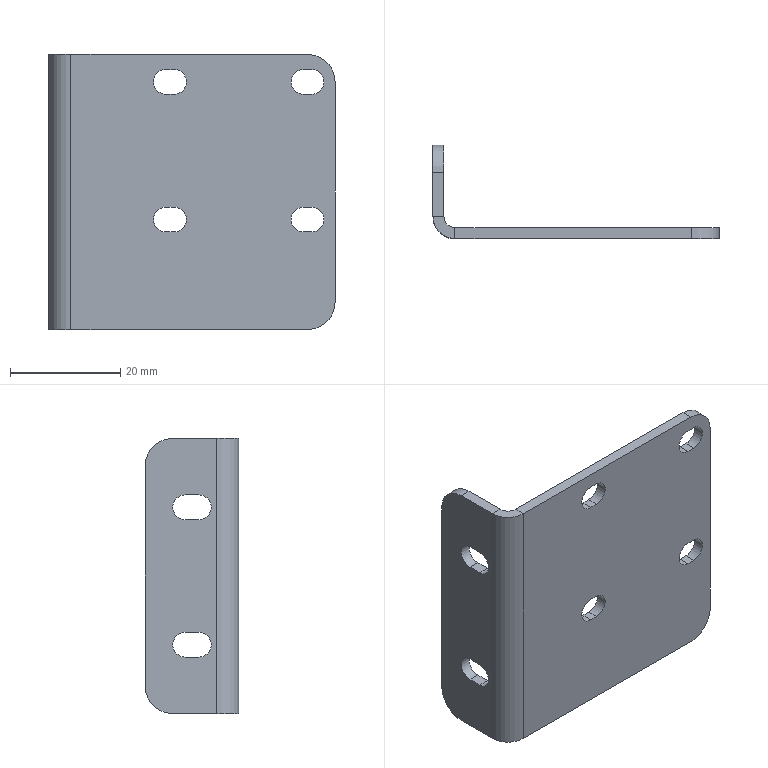Part | SolidWorks | features HoleWzd 2, Fillet 1, FlatPattern 1, SMBaseFlange 1, SheetMetal 1 | 1 solid | 42 faces | box 52 x 17 x 50 mm | volume 6238 mm3 | plane 24 | cylinder 18 | commonest cylinder face diameters 4.5 x12 10 x4 4 x1 8 x1
STEP:
#1=CARTESIAN_POINT('',(0.,-13.,50.));
#2=VERTEX_POINT('',#1);
#3=CARTESIAN_POINT('',(2.,-13.,50.));
#4=VERTEX_POINT('',#3);
#5=CARTESIAN_POINT('',(0.,-13.,50.));
#6=DIRECTION('',(1.,0.,0.));
#7=VECTOR('',#6,1000.);
#8=LINE('',#5,#7);
#9=EDGE_CURVE('',#2,#4,#8,.T.);
#10=ORIENTED_EDGE('',*,*,#9,.F.);
#11=CARTESIAN_POINT('',(4.,-17.,50.));
#12=VERTEX_POINT('',#11);
#13=CARTESIAN_POINT('',(4.,-13.,50.));
#14=DIRECTION('',(0.,0.,1.));
#15=DIRECTION('',(-1.,0.,0.));
#16=AXIS2_PLACEMENT_3D('',#13,#14,#15);
#17=CIRCLE('',#16,4.);
#18=EDGE_CURVE('',#2,#12,#17,.T.);
#19=ORIENTED_EDGE('',*,*,#18,.T.);
#20=CARTESIAN_POINT('',(4.,-15.,50.));
#21=VERTEX_POINT('',#20);
#22=CARTESIAN_POINT('',(4.,-15.,50.));
#23=DIRECTION('',(0.,-1.,0.));
#24=VECTOR('',#23,1000.);
#25=LINE('',#22,#24);
#26=EDGE_CURVE('',#21,#12,#25,.T.);
#27=ORIENTED_EDGE('',*,*,#26,.F.);
#28=CARTESIAN_POINT('',(4.,-13.,50.));
#29=DIRECTION('',(0.,0.,1.));
#30=DIRECTION('',(1.,0.,0.));
#31=AXIS2_PLACEMENT_3D('',#28,#29,#30);
#32=CIRCLE('',#31,2.);
#33=EDGE_CURVE('',#4,#21,#32,.T.);
#34=ORIENTED_EDGE('',*,*,#33,.F.);
#35=EDGE_LOOP('',(#10,#19,#27,#34));
#36=FACE_OUTER_BOUND('',#35,.T.);
#37=CARTESIAN_POINT('',(0.,-13.,50.));
#38=DIRECTION('',(0.,0.,1.));
#39=DIRECTION('',(1.,0.,0.));
#40=AXIS2_PLACEMENT_3D('',#37,#38,#39);
#41=PLANE('',#40);
#42=ADVANCED_FACE('',(#36),#41,.T.);
#43=CARTESIAN_POINT('',(2.,-5.,50.));
#44=VERTEX_POINT('',#43);
#45=CARTESIAN_POINT('',(2.,0.,50.));
#46=DIRECTION('',(0.,-1.,0.));
#47=VECTOR('',#46,1000.);
#48=LINE('',#45,#47);
#49=EDGE_CURVE('',#44,#4,#48,.T.);
#50=ORIENTED_EDGE('',*,*,#49,.F.);
#51=CARTESIAN_POINT('',(0.,-5.,50.));
#52=VERTEX_POINT('',#51);
#53=CARTESIAN_POINT('',(4.,-5.,50.));
#54=DIRECTION('',(-1.,0.,0.));
#55=VECTOR('',#54,1000.);
#56=LINE('',#53,#55);
#57=EDGE_CURVE('',#44,#52,#56,.T.);
#58=ORIENTED_EDGE('',*,*,#57,.T.);
#59=CARTESIAN_POINT('',(0.,0.,50.));
#60=DIRECTION('',(0.,-1.,0.));
#61=VECTOR('',#60,1000.);
#62=LINE('',#59,#61);
#63=EDGE_CURVE('',#52,#2,#62,.T.);
#64=ORIENTED_EDGE('',*,*,#63,.T.);
#65=ORIENTED_EDGE('',*,*,#9,.T.);
#66=EDGE_LOOP('',(#50,#58,#64,#65));
#67=FACE_OUTER_BOUND('',#66,.T.);
#68=CARTESIAN_POINT('',(4.,-15.,50.));
#69=DIRECTION('',(0.,0.,1.));
#70=DIRECTION('',(1.,0.,0.));
#71=AXIS2_PLACEMENT_3D('',#68,#69,#70);
#72=PLANE('',#71);
#73=ADVANCED_FACE('',(#67),#72,.T.);
#74=CARTESIAN_POINT('',(4.,-17.,0.));
#75=VERTEX_POINT('',#74);
#76=CARTESIAN_POINT('',(4.,-15.,0.));
#77=VERTEX_POINT('',#76);
#78=CARTESIAN_POINT('',(4.,-17.,0.));
#79=DIRECTION('',(0.,1.,0.));
#80=VECTOR('',#79,1000.);
#81=LINE('',#78,#80);
#82=EDGE_CURVE('',#75,#77,#81,.T.);
#83=ORIENTED_EDGE('',*,*,#82,.F.);
#84=CARTESIAN_POINT('',(0.,-13.,0.));
#85=VERTEX_POINT('',#84);
#86=CARTESIAN_POINT('',(4.,-13.,0.));
#87=DIRECTION('',(0.,0.,1.));
#88=DIRECTION('',(-1.,0.,0.));
#89=AXIS2_PLACEMENT_3D('',#86,#87,#88);
#90=CIRCLE('',#89,4.);
#91=EDGE_CURVE('',#85,#75,#90,.T.);
#92=ORIENTED_EDGE('',*,*,#91,.F.);
#93=CARTESIAN_POINT('',(2.,-13.,0.));
#94=VERTEX_POINT('',#93);
#95=CARTESIAN_POINT('',(2.,-13.,0.));
#96=DIRECTION('',(-1.,0.,0.));
#97=VECTOR('',#96,1000.);
#98=LINE('',#95,#97);
#99=EDGE_CURVE('',#94,#85,#98,.T.);
#100=ORIENTED_EDGE('',*,*,#99,.F.);
#101=CARTESIAN_POINT('',(4.,-13.,0.));
#102=DIRECTION('',(0.,0.,1.));
#103=DIRECTION('',(1.,0.,0.));
#104=AXIS2_PLACEMENT_3D('',#101,#102,#103);
#105=CIRCLE('',#104,2.);
#106=EDGE_CURVE('',#94,#77,#105,.T.);
#107=ORIENTED_EDGE('',*,*,#106,.T.);
#108=EDGE_LOOP('',(#83,#92,#100,#107));
#109=FACE_OUTER_BOUND('',#108,.T.);
#110=CARTESIAN_POINT('',(4.,-17.,0.));
#111=DIRECTION('',(0.,0.,-1.));
#112=DIRECTION('',(-1.,0.,0.));
#113=AXIS2_PLACEMENT_3D('',#110,#111,#112);
#114=PLANE('',#113);
#115=ADVANCED_FACE('',(#109),#114,.T.);
#116=CARTESIAN_POINT('',(47.,-15.,0.));
#117=VERTEX_POINT('',#116);
#118=CARTESIAN_POINT('',(0.,-15.,0.));
#119=DIRECTION('',(1.,0.,0.));
#120=VECTOR('',#119,1000.);
#121=LINE('',#118,#120);
#122=EDGE_CURVE('',#77,#117,#121,.T.);
#123=ORIENTED_EDGE('',*,*,#122,.T.);
#124=CARTESIAN_POINT('',(47.,-17.,0.));
#125=VERTEX_POINT('',#124);
#126=CARTESIAN_POINT('',(47.,-13.,0.));
#127=DIRECTION('',(0.,-1.,0.));
#128=VECTOR('',#127,1000.);
#129=LINE('',#126,#128);
#130=EDGE_CURVE('',#117,#125,#129,.T.);
#131=ORIENTED_EDGE('',*,*,#130,.T.);
#132=CARTESIAN_POINT('',(0.,-17.,0.));
#133=DIRECTION('',(1.,0.,0.));
#134=VECTOR('',#133,1000.);
#135=LINE('',#132,#134);
#136=EDGE_CURVE('',#75,#125,#135,.T.);
#137=ORIENTED_EDGE('',*,*,#136,.F.);
#138=ORIENTED_EDGE('',*,*,#82,.T.);
#139=EDGE_LOOP('',(#123,#131,#137,#138));
#140=FACE_OUTER_BOUND('',#139,.T.);
#141=CARTESIAN_POINT('',(2.,-13.,0.));
#142=DIRECTION('',(0.,0.,-1.));
#143=DIRECTION('',(-1.,0.,0.));
#144=AXIS2_PLACEMENT_3D('',#141,#142,#143);
#145=PLANE('',#144);
#146=ADVANCED_FACE('',(#140),#145,.T.);
#147=CARTESIAN_POINT('',(46.25,-17.,47.25));
#148=VERTEX_POINT('',#147);
#149=CARTESIAN_POINT('',(47.75,-17.,47.25));
#150=VERTEX_POINT('',#149);
#151=CARTESIAN_POINT('',(46.25,-17.,47.25));
#152=DIRECTION('',(1.,0.,0.));
#153=VECTOR('',#152,1000.);
#154=LINE('',#151,#153);
#155=EDGE_CURVE('',#148,#150,#154,.T.);
#156=ORIENTED_EDGE('',*,*,#155,.T.);
#157=CARTESIAN_POINT('',(47.75,-17.,42.75));
#158=VERTEX_POINT('',#157);
#159=CARTESIAN_POINT('',(47.75,-17.,45.));
#160=DIRECTION('',(0.,1.,0.));
#161=DIRECTION('',(0.,0.,1.));
#162=AXIS2_PLACEMENT_3D('',#159,#160,#161);
#163=CIRCLE('',#162,2.25);
#164=EDGE_CURVE('',#150,#158,#163,.T.);
#165=ORIENTED_EDGE('',*,*,#164,.T.);
#166=CARTESIAN_POINT('',(46.25,-17.,42.75));
#167=VERTEX_POINT('',#166);
#168=CARTESIAN_POINT('',(46.25,-17.,42.75));
#169=DIRECTION('',(1.,0.,0.));
#170=VECTOR('',#169,1000.);
#171=LINE('',#168,#170);
#172=EDGE_CURVE('',#167,#158,#171,.T.);
#173=ORIENTED_EDGE('',*,*,#172,.F.);
#174=CARTESIAN_POINT('',(46.25,-17.,45.));
#175=DIRECTION('',(0.,1.,0.));
#176=DIRECTION('',(0.,0.,1.));
#177=AXIS2_PLACEMENT_3D('',#174,#175,#176);
#178=CIRCLE('',#177,2.25);
#179=EDGE_CURVE('',#167,#148,#178,.T.);
#180=ORIENTED_EDGE('',*,*,#179,.T.);
#181=EDGE_LOOP('',(#156,#165,#173,#180));
#182=FACE_BOUND('',#181,.T.);
#183=CARTESIAN_POINT('',(21.25,-17.,47.25));
#184=VERTEX_POINT('',#183);
#185=CARTESIAN_POINT('',(22.75,-17.,47.25));
#186=VERTEX_POINT('',#185);
#187=CARTESIAN_POINT('',(21.25,-17.,47.25));
#188=DIRECTION('',(1.,0.,0.));
#189=VECTOR('',#188,1000.);
#190=LINE('',#187,#189);
#191=EDGE_CURVE('',#184,#186,#190,.T.);
#192=ORIENTED_EDGE('',*,*,#191,.T.);
#193=CARTESIAN_POINT('',(22.75,-17.,42.75));
#194=VERTEX_POINT('',#193);
#195=CARTESIAN_POINT('',(22.75,-17.,45.));
#196=DIRECTION('',(0.,1.,0.));
#197=DIRECTION('',(0.,0.,1.));
#198=AXIS2_PLACEMENT_3D('',#195,#196,#197);
#199=CIRCLE('',#198,2.25);
#200=EDGE_CURVE('',#186,#194,#199,.T.);
#201=ORIENTED_EDGE('',*,*,#200,.T.);
#202=CARTESIAN_POINT('',(21.25,-17.,42.75));
#203=VERTEX_POINT('',#202);
#204=CARTESIAN_POINT('',(21.25,-17.,42.75));
#205=DIRECTION('',(1.,0.,0.));
#206=VECTOR('',#205,1000.);
#207=LINE('',#204,#206);
#208=EDGE_CURVE('',#203,#194,#207,.T.);
#209=ORIENTED_EDGE('',*,*,#208,.F.);
#210=CARTESIAN_POINT('',(21.25,-17.,45.));
#211=DIRECTION('',(0.,1.,0.));
#212=DIRECTION('',(0.,0.,1.));
#213=AXIS2_PLACEMENT_3D('',#210,#211,#212);
#214=CIRCLE('',#213,2.25);
#215=EDGE_CURVE('',#203,#184,#214,.T.);
#216=ORIENTED_EDGE('',*,*,#215,.T.);
#217=EDGE_LOOP('',(#192,#201,#209,#216));
#218=FACE_BOUND('',#217,.T.);
#219=CARTESIAN_POINT('',(46.25,-17.,22.25));
#220=VERTEX_POINT('',#219);
#221=CARTESIAN_POINT('',(47.75,-17.,22.25));
#222=VERTEX_POINT('',#221);
#223=CARTESIAN_POINT('',(46.25,-17.,22.25));
#224=DIRECTION('',(1.,0.,0.));
#225=VECTOR('',#224,1000.);
#226=LINE('',#223,#225);
#227=EDGE_CURVE('',#220,#222,#226,.T.);
#228=ORIENTED_EDGE('',*,*,#227,.T.);
#229=CARTESIAN_POINT('',(47.75,-17.,17.75));
#230=VERTEX_POINT('',#229);
#231=CARTESIAN_POINT('',(47.75,-17.,20.));
#232=DIRECTION('',(0.,1.,0.));
#233=DIRECTION('',(0.,0.,1.));
#234=AXIS2_PLACEMENT_3D('',#231,#232,#233);
#235=CIRCLE('',#234,2.25);
#236=EDGE_CURVE('',#222,#230,#235,.T.);
#237=ORIENTED_EDGE('',*,*,#236,.T.);
#238=CARTESIAN_POINT('',(46.25,-17.,17.75));
#239=VERTEX_POINT('',#238);
#240=CARTESIAN_POINT('',(46.25,-17.,17.75));
#241=DIRECTION('',(1.,0.,0.));
#242=VECTOR('',#241,1000.);
#243=LINE('',#240,#242);
#244=EDGE_CURVE('',#239,#230,#243,.T.);
#245=ORIENTED_EDGE('',*,*,#244,.F.);
#246=CARTESIAN_POINT('',(46.25,-17.,20.));
#247=DIRECTION('',(0.,1.,0.));
#248=DIRECTION('',(0.,0.,1.));
#249=AXIS2_PLACEMENT_3D('',#246,#247,#248);
#250=CIRCLE('',#249,2.25);
#251=EDGE_CURVE('',#239,#220,#250,.T.);
#252=ORIENTED_EDGE('',*,*,#251,.T.);
#253=EDGE_LOOP('',(#228,#237,#245,#252));
#254=FACE_BOUND('',#253,.T.);
#255=CARTESIAN_POINT('',(21.25,-17.,22.25));
#256=VERTEX_POINT('',#255);
#257=CARTESIAN_POINT('',(22.75,-17.,22.25));
#258=VERTEX_POINT('',#257);
#259=CARTESIAN_POINT('',(21.25,-17.,22.25));
#260=DIRECTION('',(1.,0.,0.));
#261=VECTOR('',#260,1000.);
#262=LINE('',#259,#261);
#263=EDGE_CURVE('',#256,#258,#262,.T.);
#264=ORIENTED_EDGE('',*,*,#263,.T.);
#265=CARTESIAN_POINT('',(22.75,-17.,17.75));
#266=VERTEX_POINT('',#265);
#267=CARTESIAN_POINT('',(22.75,-17.,20.));
#268=DIRECTION('',(0.,1.,0.));
#269=DIRECTION('',(0.,0.,1.));
#270=AXIS2_PLACEMENT_3D('',#267,#268,#269);
#271=CIRCLE('',#270,2.25);
#272=EDGE_CURVE('',#258,#266,#271,.T.);
#273=ORIENTED_EDGE('',*,*,#272,.T.);
#274=CARTESIAN_POINT('',(21.25,-17.,17.75));
#275=VERTEX_POINT('',#274);
#276=CARTESIAN_POINT('',(21.25,-17.,17.75));
#277=DIRECTION('',(1.,0.,0.));
#278=VECTOR('',#277,1000.);
#279=LINE('',#276,#278);
#280=EDGE_CURVE('',#275,#266,#279,.T.);
#281=ORIENTED_EDGE('',*,*,#280,.F.);
#282=CARTESIAN_POINT('',(21.25,-17.,20.));
#283=DIRECTION('',(0.,1.,0.));
#284=DIRECTION('',(0.,0.,1.));
#285=AXIS2_PLACEMENT_3D('',#282,#283,#284);
#286=CIRCLE('',#285,2.25);
#287=EDGE_CURVE('',#275,#256,#286,.T.);
#288=ORIENTED_EDGE('',*,*,#287,.T.);
#289=EDGE_LOOP('',(#264,#273,#281,#288));
#290=FACE_BOUND('',#289,.T.);
#291=ORIENTED_EDGE('',*,*,#136,.T.);
#292=CARTESIAN_POINT('',(52.,-17.,5.));
#293=VERTEX_POINT('',#292);
#294=CARTESIAN_POINT('',(47.,-17.,5.));
#295=DIRECTION('',(0.,-1.,0.));
#296=DIRECTION('',(0.,0.,1.));
#297=AXIS2_PLACEMENT_3D('',#294,#295,#296);
#298=CIRCLE('',#297,5.);
#299=EDGE_CURVE('',#125,#293,#298,.T.);
#300=ORIENTED_EDGE('',*,*,#299,.T.);
#301=CARTESIAN_POINT('',(52.,-17.,45.));
#302=VERTEX_POINT('',#301);
#303=CARTESIAN_POINT('',(52.,-17.,50.));
#304=DIRECTION('',(0.,0.,-1.));
#305=VECTOR('',#304,1000.);
#306=LINE('',#303,#305);
#307=EDGE_CURVE('',#302,#293,#306,.T.);
#308=ORIENTED_EDGE('',*,*,#307,.F.);
#309=CARTESIAN_POINT('',(47.,-17.,50.));
#310=VERTEX_POINT('',#309);
#311=CARTESIAN_POINT('',(47.,-17.,45.));
#312=DIRECTION('',(0.,-1.,0.));
#313=DIRECTION('',(0.,0.,1.));
#314=AXIS2_PLACEMENT_3D('',#311,#312,#313);
#315=CIRCLE('',#314,5.);
#316=EDGE_CURVE('',#302,#310,#315,.T.);
#317=ORIENTED_EDGE('',*,*,#316,.T.);
#318=CARTESIAN_POINT('',(0.,-17.,50.));
#319=DIRECTION('',(1.,0.,0.));
#320=VECTOR('',#319,1000.);
#321=LINE('',#318,#320);
#322=EDGE_CURVE('',#12,#310,#321,.T.);
#323=ORIENTED_EDGE('',*,*,#322,.F.);
#324=CARTESIAN_POINT('',(4.,-17.,50.));
#325=DIRECTION('',(0.,0.,-1.));
#326=VECTOR('',#325,1000.);
#327=LINE('',#324,#326);
#328=EDGE_CURVE('',#12,#75,#327,.T.);
#329=ORIENTED_EDGE('',*,*,#328,.T.);
#330=EDGE_LOOP('',(#291,#300,#308,#317,#323,#329));
#331=FACE_OUTER_BOUND('',#330,.T.);
#332=CARTESIAN_POINT('',(0.,-17.,50.));
#333=DIRECTION('',(0.,1.,0.));
#334=DIRECTION('',(0.,0.,1.));
#335=AXIS2_PLACEMENT_3D('',#332,#333,#334);
#336=PLANE('',#335);
#337=ADVANCED_FACE('',(#182,#218,#254,#290,#331),#336,.F.);
#338=ORIENTED_EDGE('',*,*,#307,.T.);
#339=CARTESIAN_POINT('',(52.,-15.,5.));
#340=VERTEX_POINT('',#339);
#341=CARTESIAN_POINT('',(52.,-15.,5.));
#342=DIRECTION('',(0.,1.,0.));
#343=VECTOR('',#342,1000.);
#344=LINE('',#341,#343);
#345=EDGE_CURVE('',#293,#340,#344,.T.);
#346=ORIENTED_EDGE('',*,*,#345,.T.);
#347=CARTESIAN_POINT('',(52.,-15.,45.));
#348=VERTEX_POINT('',#347);
#349=CARTESIAN_POINT('',(52.,-15.,50.));
#350=DIRECTION('',(0.,0.,-1.));
#351=VECTOR('',#350,1000.);
#352=LINE('',#349,#351);
#353=EDGE_CURVE('',#348,#340,#352,.T.);
#354=ORIENTED_EDGE('',*,*,#353,.F.);
#355=CARTESIAN_POINT('',(52.,-15.,45.));
#356=DIRECTION('',(0.,-1.,0.));
#357=VECTOR('',#356,1000.);
#358=LINE('',#355,#357);
#359=EDGE_CURVE('',#348,#302,#358,.T.);
#360=ORIENTED_EDGE('',*,*,#359,.T.);
#361=EDGE_LOOP('',(#338,#346,#354,#360));
#362=FACE_OUTER_BOUND('',#361,.T.);
#363=CARTESIAN_POINT('',(52.,-15.,50.));
#364=DIRECTION('',(1.,0.,0.));
#365=DIRECTION('',(0.,0.,-1.));
#366=AXIS2_PLACEMENT_3D('',#363,#364,#365);
#367=PLANE('',#366);
#368=ADVANCED_FACE('',(#362),#367,.T.);
#369=CARTESIAN_POINT('',(46.25,-15.,47.25));
#370=VERTEX_POINT('',#369);
#371=CARTESIAN_POINT('',(47.75,-15.,47.25));
#372=VERTEX_POINT('',#371);
#373=CARTESIAN_POINT('',(46.25,-15.,47.25));
#374=DIRECTION('',(1.,0.,0.));
#375=VECTOR('',#374,1000.);
#376=LINE('',#373,#375);
#377=EDGE_CURVE('',#370,#372,#376,.T.);
#378=ORIENTED_EDGE('',*,*,#377,.F.);
#379=CARTESIAN_POINT('',(46.25,-15.,42.75));
#380=VERTEX_POINT('',#379);
#381=CARTESIAN_POINT('',(46.25,-15.,45.));
#382=DIRECTION('',(0.,1.,0.));
#383=DIRECTION('',(0.,0.,1.));
#384=AXIS2_PLACEMENT_3D('',#381,#382,#383);
#385=CIRCLE('',#384,2.25);
#386=EDGE_CURVE('',#380,#370,#385,.T.);
#387=ORIENTED_EDGE('',*,*,#386,.F.);
#388=CARTESIAN_POINT('',(47.75,-15.,42.75));
#389=VERTEX_POINT('',#388);
#390=CARTESIAN_POINT('',(46.25,-15.,42.75));
#391=DIRECTION('',(1.,0.,0.));
#392=VECTOR('',#391,1000.);
#393=LINE('',#390,#392);
#394=EDGE_CURVE('',#380,#389,#393,.T.);
#395=ORIENTED_EDGE('',*,*,#394,.T.);
#396=CARTESIAN_POINT('',(47.75,-15.,45.));
#397=DIRECTION('',(0.,1.,0.));
#398=DIRECTION('',(0.,0.,1.));
#399=AXIS2_PLACEMENT_3D('',#396,#397,#398);
#400=CIRCLE('',#399,2.25);
#401=EDGE_CURVE('',#372,#389,#400,.T.);
#402=ORIENTED_EDGE('',*,*,#401,.F.);
#403=EDGE_LOOP('',(#378,#387,#395,#402));
#404=FACE_BOUND('',#403,.T.);
#405=CARTESIAN_POINT('',(22.75,-15.,47.25));
#406=VERTEX_POINT('',#405);
#407=CARTESIAN_POINT('',(22.75,-15.,42.75));
#408=VERTEX_POINT('',#407);
#409=CARTESIAN_POINT('',(22.75,-15.,45.));
#410=DIRECTION('',(0.,1.,0.));
#411=DIRECTION('',(0.,0.,1.));
#412=AXIS2_PLACEMENT_3D('',#409,#410,#411);
#413=CIRCLE('',#412,2.25);
#414=EDGE_CURVE('',#406,#408,#413,.T.);
#415=ORIENTED_EDGE('',*,*,#414,.F.);
#416=CARTESIAN_POINT('',(21.25,-15.,47.25));
#417=VERTEX_POINT('',#416);
#418=CARTESIAN_POINT('',(21.25,-15.,47.25));
#419=DIRECTION('',(1.,0.,0.));
#420=VECTOR('',#419,1000.);
#421=LINE('',#418,#420);
#422=EDGE_CURVE('',#417,#406,#421,.T.);
#423=ORIENTED_EDGE('',*,*,#422,.F.);
#424=CARTESIAN_POINT('',(21.25,-15.,42.75));
#425=VERTEX_POINT('',#424);
#426=CARTESIAN_POINT('',(21.25,-15.,45.));
#427=DIRECTION('',(0.,1.,0.));
#428=DIRECTION('',(0.,0.,1.));
#429=AXIS2_PLACEMENT_3D('',#426,#427,#428);
#430=CIRCLE('',#429,2.25);
#431=EDGE_CURVE('',#425,#417,#430,.T.);
#432=ORIENTED_EDGE('',*,*,#431,.F.);
#433=CARTESIAN_POINT('',(21.25,-15.,42.75));
#434=DIRECTION('',(1.,0.,0.));
#435=VECTOR('',#434,1000.);
#436=LINE('',#433,#435);
#437=EDGE_CURVE('',#425,#408,#436,.T.);
#438=ORIENTED_EDGE('',*,*,#437,.T.);
#439=EDGE_LOOP('',(#415,#423,#432,#438));
#440=FACE_BOUND('',#439,.T.);
#441=CARTESIAN_POINT('',(47.75,-15.,22.25));
#442=VERTEX_POINT('',#441);
#443=CARTESIAN_POINT('',(47.75,-15.,17.75));
#444=VERTEX_POINT('',#443);
#445=CARTESIAN_POINT('',(47.75,-15.,20.));
#446=DIRECTION('',(0.,1.,0.));
#447=DIRECTION('',(0.,0.,1.));
#448=AXIS2_PLACEMENT_3D('',#445,#446,#447);
#449=CIRCLE('',#448,2.25);
#450=EDGE_CURVE('',#442,#444,#449,.T.);
#451=ORIENTED_EDGE('',*,*,#450,.F.);
#452=CARTESIAN_POINT('',(46.25,-15.,22.25));
#453=VERTEX_POINT('',#452);
#454=CARTESIAN_POINT('',(46.25,-15.,22.25));
#455=DIRECTION('',(1.,0.,0.));
#456=VECTOR('',#455,1000.);
#457=LINE('',#454,#456);
#458=EDGE_CURVE('',#453,#442,#457,.T.);
#459=ORIENTED_EDGE('',*,*,#458,.F.);
#460=CARTESIAN_POINT('',(46.25,-15.,17.75));
#461=VERTEX_POINT('',#460);
#462=CARTESIAN_POINT('',(46.25,-15.,20.));
#463=DIRECTION('',(0.,1.,0.));
#464=DIRECTION('',(0.,0.,1.));
#465=AXIS2_PLACEMENT_3D('',#462,#463,#464);
#466=CIRCLE('',#465,2.25);
#467=EDGE_CURVE('',#461,#453,#466,.T.);
#468=ORIENTED_EDGE('',*,*,#467,.F.);
#469=CARTESIAN_POINT('',(46.25,-15.,17.75));
#470=DIRECTION('',(1.,0.,0.));
#471=VECTOR('',#470,1000.);
#472=LINE('',#469,#471);
#473=EDGE_CURVE('',#461,#444,#472,.T.);
#474=ORIENTED_EDGE('',*,*,#473,.T.);
#475=EDGE_LOOP('',(#451,#459,#468,#474));
#476=FACE_BOUND('',#475,.T.);
#477=CARTESIAN_POINT('',(22.75,-15.,22.25));
#478=VERTEX_POINT('',#477);
#479=CARTESIAN_POINT('',(22.75,-15.,17.75));
#480=VERTEX_POINT('',#479);
#481=CARTESIAN_POINT('',(22.75,-15.,20.));
#482=DIRECTION('',(0.,1.,0.));
#483=DIRECTION('',(0.,0.,1.));
#484=AXIS2_PLACEMENT_3D('',#481,#482,#483);
#485=CIRCLE('',#484,2.25);
#486=EDGE_CURVE('',#478,#480,#485,.T.);
#487=ORIENTED_EDGE('',*,*,#486,.F.);
#488=CARTESIAN_POINT('',(21.25,-15.,22.25));
#489=VERTEX_POINT('',#488);
#490=CARTESIAN_POINT('',(21.25,-15.,22.25));
#491=DIRECTION('',(1.,0.,0.));
#492=VECTOR('',#491,1000.);
#493=LINE('',#490,#492);
#494=EDGE_CURVE('',#489,#478,#493,.T.);
#495=ORIENTED_EDGE('',*,*,#494,.F.);
#496=CARTESIAN_POINT('',(21.25,-15.,17.75));
#497=VERTEX_POINT('',#496);
#498=CARTESIAN_POINT('',(21.25,-15.,20.));
#499=DIRECTION('',(0.,1.,0.));
#500=DIRECTION('',(0.,0.,1.));
#501=AXIS2_PLACEMENT_3D('',#498,#499,#500);
#502=CIRCLE('',#501,2.25);
#503=EDGE_CURVE('',#497,#489,#502,.T.);
#504=ORIENTED_EDGE('',*,*,#503,.F.);
#505=CARTESIAN_POINT('',(21.25,-15.,17.75));
#506=DIRECTION('',(1.,0.,0.));
#507=VECTOR('',#506,1000.);
#508=LINE('',#505,#507);
#509=EDGE_CURVE('',#497,#480,#508,.T.);
#510=ORIENTED_EDGE('',*,*,#509,.T.);
#511=EDGE_LOOP('',(#487,#495,#504,#510));
#512=FACE_BOUND('',#511,.T.);
#513=ORIENTED_EDGE('',*,*,#353,.T.);
#514=CARTESIAN_POINT('',(47.,-15.,5.));
#515=DIRECTION('',(0.,1.,0.));
#516=DIRECTION('',(0.,0.,1.));
#517=AXIS2_PLACEMENT_3D('',#514,#515,#516);
#518=CIRCLE('',#517,5.);
#519=EDGE_CURVE('',#340,#117,#518,.T.);
#520=ORIENTED_EDGE('',*,*,#519,.T.);
#521=ORIENTED_EDGE('',*,*,#122,.F.);
#522=CARTESIAN_POINT('',(4.,-15.,50.));
#523=DIRECTION('',(0.,0.,-1.));
#524=VECTOR('',#523,1000.);
#525=LINE('',#522,#524);
#526=EDGE_CURVE('',#21,#77,#525,.T.);
#527=ORIENTED_EDGE('',*,*,#526,.F.);
#528=CARTESIAN_POINT('',(47.,-15.,50.));
#529=VERTEX_POINT('',#528);
#530=CARTESIAN_POINT('',(0.,-15.,50.));
#531=DIRECTION('',(1.,0.,0.));
#532=VECTOR('',#531,1000.);
#533=LINE('',#530,#532);
#534=EDGE_CURVE('',#21,#529,#533,.T.);
#535=ORIENTED_EDGE('',*,*,#534,.T.);
#536=CARTESIAN_POINT('',(47.,-15.,45.));
#537=DIRECTION('',(0.,1.,0.));
#538=DIRECTION('',(0.,0.,1.));
#539=AXIS2_PLACEMENT_3D('',#536,#537,#538);
#540=CIRCLE('',#539,5.);
#541=EDGE_CURVE('',#529,#348,#540,.T.);
#542=ORIENTED_EDGE('',*,*,#541,.T.);
#543=EDGE_LOOP('',(#513,#520,#521,#527,#535,#542));
#544=FACE_OUTER_BOUND('',#543,.T.);
#545=CARTESIAN_POINT('',(0.,-15.,50.));
#546=DIRECTION('',(0.,1.,0.));
#547=DIRECTION('',(0.,0.,1.));
#548=AXIS2_PLACEMENT_3D('',#545,#546,#547);
#549=PLANE('',#548);
#550=ADVANCED_FACE('',(#404,#440,#476,#512,#544),#549,.T.);
#551=ORIENTED_EDGE('',*,*,#106,.F.);
#552=CARTESIAN_POINT('',(2.,-13.,50.));
#553=DIRECTION('',(0.,0.,-1.));
#554=VECTOR('',#553,1000.);
#555=LINE('',#552,#554);
#556=EDGE_CURVE('',#4,#94,#555,.T.);
#557=ORIENTED_EDGE('',*,*,#556,.F.);
#558=ORIENTED_EDGE('',*,*,#33,.T.);
#559=ORIENTED_EDGE('',*,*,#526,.T.);
#560=EDGE_LOOP('',(#551,#557,#558,#559));
#561=FACE_OUTER_BOUND('',#560,.T.);
#562=CARTESIAN_POINT('',(4.,-13.,50.));
#563=DIRECTION('',(0.,0.,-1.));
#564=DIRECTION('',(-1.,0.,0.));
#565=AXIS2_PLACEMENT_3D('',#562,#563,#564);
#566=CYLINDRICAL_SURFACE('',#565,2.);
#567=ADVANCED_FACE('',(#561),#566,.F.);
#568=CARTESIAN_POINT('',(2.,-9.75,14.75));
#569=VERTEX_POINT('',#568);
#570=CARTESIAN_POINT('',(2.,-9.75,10.25));
#571=VERTEX_POINT('',#570);
#572=CARTESIAN_POINT('',(2.,-9.75,12.5));
#573=DIRECTION('',(1.,0.,0.));
#574=DIRECTION('',(0.,0.,-1.));
#575=AXIS2_PLACEMENT_3D('',#572,#573,#574);
#576=CIRCLE('',#575,2.25);
#577=EDGE_CURVE('',#569,#571,#576,.T.);
#578=ORIENTED_EDGE('',*,*,#577,.F.);
#579=CARTESIAN_POINT('',(2.,-7.25,14.75));
#580=VERTEX_POINT('',#579);
#581=CARTESIAN_POINT('',(2.,-9.75,14.75));
#582=DIRECTION('',(0.,1.,0.));
#583=VECTOR('',#582,1000.);
#584=LINE('',#581,#583);
#585=EDGE_CURVE('',#569,#580,#584,.T.);
#586=ORIENTED_EDGE('',*,*,#585,.T.);
#587=CARTESIAN_POINT('',(2.,-7.25,10.25));
#588=VERTEX_POINT('',#587);
#589=CARTESIAN_POINT('',(2.,-7.25,12.5));
#590=DIRECTION('',(1.,0.,0.));
#591=DIRECTION('',(0.,0.,-1.));
#592=AXIS2_PLACEMENT_3D('',#589,#590,#591);
#593=CIRCLE('',#592,2.25);
#594=EDGE_CURVE('',#588,#580,#593,.T.);
#595=ORIENTED_EDGE('',*,*,#594,.F.);
#596=CARTESIAN_POINT('',(2.,-9.75,10.25));
#597=DIRECTION('',(0.,1.,0.));
#598=VECTOR('',#597,1000.);
#599=LINE('',#596,#598);
#600=EDGE_CURVE('',#571,#588,#599,.T.);
#601=ORIENTED_EDGE('',*,*,#600,.F.);
#602=EDGE_LOOP('',(#578,#586,#595,#601));
#603=FACE_BOUND('',#602,.T.);
#604=CARTESIAN_POINT('',(2.,-9.75,35.25));
#605=VERTEX_POINT('',#604);
#606=CARTESIAN_POINT('',(2.,-7.25,35.25));
#607=VERTEX_POINT('',#606);
#608=CARTESIAN_POINT('',(2.,-9.75,35.25));
#609=DIRECTION('',(0.,1.,0.));
#610=VECTOR('',#609,1000.);
#611=LINE('',#608,#610);
#612=EDGE_CURVE('',#605,#607,#611,.T.);
#613=ORIENTED_EDGE('',*,*,#612,.F.);
#614=CARTESIAN_POINT('',(2.,-9.75,39.75));
#615=VERTEX_POINT('',#614);
#616=CARTESIAN_POINT('',(2.,-9.75,37.5));
#617=DIRECTION('',(1.,0.,0.));
#618=DIRECTION('',(0.,0.,-1.));
#619=AXIS2_PLACEMENT_3D('',#616,#617,#618);
#620=CIRCLE('',#619,2.25);
#621=EDGE_CURVE('',#615,#605,#620,.T.);
#622=ORIENTED_EDGE('',*,*,#621,.F.);
#623=CARTESIAN_POINT('',(2.,-7.25,39.75));
#624=VERTEX_POINT('',#623);
#625=CARTESIAN_POINT('',(2.,-9.75,39.75));
#626=DIRECTION('',(0.,1.,0.));
#627=VECTOR('',#626,1000.);
#628=LINE('',#625,#627);
#629=EDGE_CURVE('',#615,#624,#628,.T.);
#630=ORIENTED_EDGE('',*,*,#629,.T.);
#631=CARTESIAN_POINT('',(2.,-7.25,37.5));
#632=DIRECTION('',(1.,0.,0.));
#633=DIRECTION('',(0.,0.,-1.));
#634=AXIS2_PLACEMENT_3D('',#631,#632,#633);
#635=CIRCLE('',#634,2.25);
#636=EDGE_CURVE('',#607,#624,#635,.T.);
#637=ORIENTED_EDGE('',*,*,#636,.F.);
#638=EDGE_LOOP('',(#613,#622,#630,#637));
#639=FACE_BOUND('',#638,.T.);
#640=CARTESIAN_POINT('',(2.,0.,45.));
#641=VERTEX_POINT('',#640);
#642=CARTESIAN_POINT('',(2.,0.,5.));
#643=VERTEX_POINT('',#642);
#644=CARTESIAN_POINT('',(2.,0.,50.));
#645=DIRECTION('',(0.,0.,-1.));
#646=VECTOR('',#645,1000.);
#647=LINE('',#644,#646);
#648=EDGE_CURVE('',#641,#643,#647,.T.);
#649=ORIENTED_EDGE('',*,*,#648,.F.);
#650=CARTESIAN_POINT('',(2.,-5.,45.));
#651=DIRECTION('',(1.,0.,0.));
#652=DIRECTION('',(0.,1.,0.));
#653=AXIS2_PLACEMENT_3D('',#650,#651,#652);
#654=CIRCLE('',#653,5.);
#655=EDGE_CURVE('',#641,#44,#654,.T.);
#656=ORIENTED_EDGE('',*,*,#655,.T.);
#657=ORIENTED_EDGE('',*,*,#49,.T.);
#658=ORIENTED_EDGE('',*,*,#556,.T.);
#659=CARTESIAN_POINT('',(2.,-5.,0.));
#660=VERTEX_POINT('',#659);
#661=CARTESIAN_POINT('',(2.,0.,0.));
#662=DIRECTION('',(0.,-1.,0.));
#663=VECTOR('',#662,1000.);
#664=LINE('',#661,#663);
#665=EDGE_CURVE('',#660,#94,#664,.T.);
#666=ORIENTED_EDGE('',*,*,#665,.F.);
#667=CARTESIAN_POINT('',(2.,-5.,5.));
#668=DIRECTION('',(1.,0.,0.));
#669=DIRECTION('',(0.,1.,0.));
#670=AXIS2_PLACEMENT_3D('',#667,#668,#669);
#671=CIRCLE('',#670,5.);
#672=EDGE_CURVE('',#660,#643,#671,.T.);
#673=ORIENTED_EDGE('',*,*,#672,.T.);
#674=EDGE_LOOP('',(#649,#656,#657,#658,#666,#673));
#675=FACE_OUTER_BOUND('',#674,.T.);
#676=CARTESIAN_POINT('',(2.,0.,50.));
#677=DIRECTION('',(1.,0.,0.));
#678=DIRECTION('',(0.,1.,0.));
#679=AXIS2_PLACEMENT_3D('',#676,#677,#678);
#680=PLANE('',#679);
#681=ADVANCED_FACE('',(#603,#639,#675),#680,.T.);
#682=CARTESIAN_POINT('',(0.,0.,45.));
#683=VERTEX_POINT('',#682);
#684=CARTESIAN_POINT('',(0.,0.,5.));
#685=VERTEX_POINT('',#684);
#686=CARTESIAN_POINT('',(0.,0.,50.));
#687=DIRECTION('',(0.,0.,-1.));
#688=VECTOR('',#687,1000.);
#689=LINE('',#686,#688);
#690=EDGE_CURVE('',#683,#685,#689,.T.);
#691=ORIENTED_EDGE('',*,*,#690,.F.);
#692=CARTESIAN_POINT('',(0.,0.,45.));
#693=DIRECTION('',(1.,0.,0.));
#694=VECTOR('',#693,1000.);
#695=LINE('',#692,#694);
#696=EDGE_CURVE('',#683,#641,#695,.T.);
#697=ORIENTED_EDGE('',*,*,#696,.T.);
#698=ORIENTED_EDGE('',*,*,#648,.T.);
#699=CARTESIAN_POINT('',(0.,0.,5.));
#700=DIRECTION('',(-1.,0.,0.));
#701=VECTOR('',#700,1000.);
#702=LINE('',#699,#701);
#703=EDGE_CURVE('',#643,#685,#702,.T.);
#704=ORIENTED_EDGE('',*,*,#703,.T.);
#705=EDGE_LOOP('',(#691,#697,#698,#704));
#706=FACE_OUTER_BOUND('',#705,.T.);
#707=CARTESIAN_POINT('',(0.,0.,50.));
#708=DIRECTION('',(0.,1.,0.));
#709=DIRECTION('',(-1.,0.,0.));
#710=AXIS2_PLACEMENT_3D('',#707,#708,#709);
#711=PLANE('',#710);
#712=ADVANCED_FACE('',(#706),#711,.T.);
#713=CARTESIAN_POINT('',(0.,-7.25,14.75));
#714=VERTEX_POINT('',#713);
#715=CARTESIAN_POINT('',(0.,-9.75,14.75));
#716=VERTEX_POINT('',#715);
#717=CARTESIAN_POINT('',(0.,0.,14.75));
#718=DIRECTION('',(0.,-1.,0.));
#719=VECTOR('',#718,1000.);
#720=LINE('',#717,#719);
#721=EDGE_CURVE('',#714,#716,#720,.T.);
#722=ORIENTED_EDGE('',*,*,#721,.T.);
#723=CARTESIAN_POINT('',(0.,-9.75,10.25));
#724=VERTEX_POINT('',#723);
#725=CARTESIAN_POINT('',(0.,-9.75,12.5));
#726=DIRECTION('',(1.,0.,0.));
#727=DIRECTION('',(0.,1.,0.));
#728=AXIS2_PLACEMENT_3D('',#725,#726,#727);
#729=CIRCLE('',#728,2.25);
#730=EDGE_CURVE('',#716,#724,#729,.T.);
#731=ORIENTED_EDGE('',*,*,#730,.T.);
#732=CARTESIAN_POINT('',(0.,-7.25,10.25));
#733=VERTEX_POINT('',#732);
#734=CARTESIAN_POINT('',(0.,0.,10.25));
#735=DIRECTION('',(0.,1.,0.));
#736=VECTOR('',#735,1000.);
#737=LINE('',#734,#736);
#738=EDGE_CURVE('',#724,#733,#737,.T.);
#739=ORIENTED_EDGE('',*,*,#738,.T.);
#740=CARTESIAN_POINT('',(0.,-7.25,12.5));
#741=DIRECTION('',(1.,0.,0.));
#742=DIRECTION('',(0.,1.,0.));
#743=AXIS2_PLACEMENT_3D('',#740,#741,#742);
#744=CIRCLE('',#743,2.25);
#745=EDGE_CURVE('',#733,#714,#744,.T.);
#746=ORIENTED_EDGE('',*,*,#745,.T.);
#747=EDGE_LOOP('',(#722,#731,#739,#746));
#748=FACE_BOUND('',#747,.T.);
#749=CARTESIAN_POINT('',(0.,-7.25,35.25));
#750=VERTEX_POINT('',#749);
#751=CARTESIAN_POINT('',(0.,-7.25,39.75));
#752=VERTEX_POINT('',#751);
#753=CARTESIAN_POINT('',(0.,-7.25,37.5));
#754=DIRECTION('',(1.,0.,0.));
#755=DIRECTION('',(0.,1.,0.));
#756=AXIS2_PLACEMENT_3D('',#753,#754,#755);
#757=CIRCLE('',#756,2.25);
#758=EDGE_CURVE('',#750,#752,#757,.T.);
#759=ORIENTED_EDGE('',*,*,#758,.T.);
#760=CARTESIAN_POINT('',(0.,-9.75,39.75));
#761=VERTEX_POINT('',#760);
#762=CARTESIAN_POINT('',(0.,0.,39.75));
#763=DIRECTION('',(0.,-1.,0.));
#764=VECTOR('',#763,1000.);
#765=LINE('',#762,#764);
#766=EDGE_CURVE('',#752,#761,#765,.T.);
#767=ORIENTED_EDGE('',*,*,#766,.T.);
#768=CARTESIAN_POINT('',(0.,-9.75,35.25));
#769=VERTEX_POINT('',#768);
#770=CARTESIAN_POINT('',(0.,-9.75,37.5));
#771=DIRECTION('',(1.,0.,0.));
#772=DIRECTION('',(0.,1.,0.));
#773=AXIS2_PLACEMENT_3D('',#770,#771,#772);
#774=CIRCLE('',#773,2.25);
#775=EDGE_CURVE('',#761,#769,#774,.T.);
#776=ORIENTED_EDGE('',*,*,#775,.T.);
#777=CARTESIAN_POINT('',(0.,0.,35.25));
#778=DIRECTION('',(0.,1.,0.));
#779=VECTOR('',#778,1000.);
#780=LINE('',#777,#779);
#781=EDGE_CURVE('',#769,#750,#780,.T.);
#782=ORIENTED_EDGE('',*,*,#781,.T.);
#783=EDGE_LOOP('',(#759,#767,#776,#782));
#784=FACE_BOUND('',#783,.T.);
#785=ORIENTED_EDGE('',*,*,#63,.F.);
#786=CARTESIAN_POINT('',(0.,-5.,45.));
#787=DIRECTION('',(-1.,0.,0.));
#788=DIRECTION('',(0.,1.,0.));
#789=AXIS2_PLACEMENT_3D('',#786,#787,#788);
#790=CIRCLE('',#789,5.);
#791=EDGE_CURVE('',#52,#683,#790,.T.);
#792=ORIENTED_EDGE('',*,*,#791,.T.);
#793=ORIENTED_EDGE('',*,*,#690,.T.);
#794=CARTESIAN_POINT('',(0.,-5.,0.));
#795=VERTEX_POINT('',#794);
#796=CARTESIAN_POINT('',(0.,-5.,5.));
#797=DIRECTION('',(-1.,0.,0.));
#798=DIRECTION('',(0.,1.,0.));
#799=AXIS2_PLACEMENT_3D('',#796,#797,#798);
#800=CIRCLE('',#799,5.);
#801=EDGE_CURVE('',#685,#795,#800,.T.);
#802=ORIENTED_EDGE('',*,*,#801,.T.);
#803=CARTESIAN_POINT('',(0.,0.,0.));
#804=DIRECTION('',(0.,-1.,0.));
#805=VECTOR('',#804,1000.);
#806=LINE('',#803,#805);
#807=EDGE_CURVE('',#795,#85,#806,.T.);
#808=ORIENTED_EDGE('',*,*,#807,.T.);
#809=CARTESIAN_POINT('',(0.,-13.,50.));
#810=DIRECTION('',(0.,0.,-1.));
#811=VECTOR('',#810,1000.);
#812=LINE('',#809,#811);
#813=EDGE_CURVE('',#2,#85,#812,.T.);
#814=ORIENTED_EDGE('',*,*,#813,.F.);
#815=EDGE_LOOP('',(#785,#792,#793,#802,#808,#814));
#816=FACE_OUTER_BOUND('',#815,.T.);
#817=CARTESIAN_POINT('',(0.,0.,50.));
#818=DIRECTION('',(1.,0.,0.));
#819=DIRECTION('',(0.,1.,0.));
#820=AXIS2_PLACEMENT_3D('',#817,#818,#819);
#821=PLANE('',#820);
#822=ADVANCED_FACE('',(#748,#784,#816),#821,.F.);
#823=ORIENTED_EDGE('',*,*,#91,.T.);
#824=ORIENTED_EDGE('',*,*,#328,.F.);
#825=ORIENTED_EDGE('',*,*,#18,.F.);
#826=ORIENTED_EDGE('',*,*,#813,.T.);
#827=EDGE_LOOP('',(#823,#824,#825,#826));
#828=FACE_OUTER_BOUND('',#827,.T.);
#829=CARTESIAN_POINT('',(4.,-13.,50.));
#830=DIRECTION('',(0.,0.,-1.));
#831=DIRECTION('',(-1.,0.,0.));
#832=AXIS2_PLACEMENT_3D('',#829,#830,#831);
#833=CYLINDRICAL_SURFACE('',#832,4.);
#834=ADVANCED_FACE('',(#828),#833,.T.);
#835=ORIENTED_EDGE('',*,*,#322,.T.);
#836=CARTESIAN_POINT('',(47.,-13.,50.));
#837=DIRECTION('',(0.,1.,0.));
#838=VECTOR('',#837,1000.);
#839=LINE('',#836,#838);
#840=EDGE_CURVE('',#310,#529,#839,.T.);
#841=ORIENTED_EDGE('',*,*,#840,.T.);
#842=ORIENTED_EDGE('',*,*,#534,.F.);
#843=ORIENTED_EDGE('',*,*,#26,.T.);
#844=EDGE_LOOP('',(#835,#841,#842,#843));
#845=FACE_OUTER_BOUND('',#844,.T.);
#846=CARTESIAN_POINT('',(4.,-13.,50.));
#847=DIRECTION('',(0.,0.,1.));
#848=DIRECTION('',(1.,0.,0.));
#849=AXIS2_PLACEMENT_3D('',#846,#847,#848);
#850=PLANE('',#849);
#851=ADVANCED_FACE('',(#845),#850,.T.);
#852=ORIENTED_EDGE('',*,*,#807,.F.);
#853=CARTESIAN_POINT('',(2.,-5.,0.));
#854=DIRECTION('',(1.,0.,0.));
#855=VECTOR('',#854,1000.);
#856=LINE('',#853,#855);
#857=EDGE_CURVE('',#795,#660,#856,.T.);
#858=ORIENTED_EDGE('',*,*,#857,.T.);
#859=ORIENTED_EDGE('',*,*,#665,.T.);
#860=ORIENTED_EDGE('',*,*,#99,.T.);
#861=EDGE_LOOP('',(#852,#858,#859,#860));
#862=FACE_OUTER_BOUND('',#861,.T.);
#863=CARTESIAN_POINT('',(4.,-13.,0.));
#864=DIRECTION('',(0.,0.,1.));
#865=DIRECTION('',(1.,0.,0.));
#866=AXIS2_PLACEMENT_3D('',#863,#864,#865);
#867=PLANE('',#866);
#868=ADVANCED_FACE('',(#862),#867,.F.);
#869=ORIENTED_EDGE('',*,*,#272,.F.);
#870=CARTESIAN_POINT('',(22.75,-15.,22.25));
#871=DIRECTION('',(0.,-1.,0.));
#872=VECTOR('',#871,1000.);
#873=LINE('',#870,#872);
#874=EDGE_CURVE('',#478,#258,#873,.T.);
#875=ORIENTED_EDGE('',*,*,#874,.F.);
#876=ORIENTED_EDGE('',*,*,#486,.T.);
#877=CARTESIAN_POINT('',(22.75,-15.,17.75));
#878=DIRECTION('',(0.,1.,0.));
#879=VECTOR('',#878,1000.);
#880=LINE('',#877,#879);
#881=EDGE_CURVE('',#266,#480,#880,.T.);
#882=ORIENTED_EDGE('',*,*,#881,.F.);
#883=EDGE_LOOP('',(#869,#875,#876,#882));
#884=FACE_OUTER_BOUND('',#883,.T.);
#885=CARTESIAN_POINT('',(22.75,-15.,20.));
#886=DIRECTION('',(0.,1.,0.));
#887=DIRECTION('',(0.,0.,1.));
#888=AXIS2_PLACEMENT_3D('',#885,#886,#887);
#889=CYLINDRICAL_SURFACE('',#888,2.25);
#890=ADVANCED_FACE('',(#884),#889,.F.);
#891=ORIENTED_EDGE('',*,*,#503,.T.);
#892=CARTESIAN_POINT('',(21.25,-15.,22.25));
#893=DIRECTION('',(0.,1.,0.));
#894=VECTOR('',#893,1000.);
#895=LINE('',#892,#894);
#896=EDGE_CURVE('',#256,#489,#895,.T.);
#897=ORIENTED_EDGE('',*,*,#896,.F.);
#898=ORIENTED_EDGE('',*,*,#287,.F.);
#899=CARTESIAN_POINT('',(21.25,-15.,17.75));
#900=DIRECTION('',(0.,-1.,0.));
#901=VECTOR('',#900,1000.);
#902=LINE('',#899,#901);
#903=EDGE_CURVE('',#497,#275,#902,.T.);
#904=ORIENTED_EDGE('',*,*,#903,.F.);
#905=EDGE_LOOP('',(#891,#897,#898,#904));
#906=FACE_OUTER_BOUND('',#905,.T.);
#907=CARTESIAN_POINT('',(21.25,-15.,20.));
#908=DIRECTION('',(0.,1.,0.));
#909=DIRECTION('',(0.,0.,1.));
#910=AXIS2_PLACEMENT_3D('',#907,#908,#909);
#911=CYLINDRICAL_SURFACE('',#910,2.25);
#912=ADVANCED_FACE('',(#906),#911,.F.);
#913=ORIENTED_EDGE('',*,*,#881,.T.);
#914=ORIENTED_EDGE('',*,*,#509,.F.);
#915=ORIENTED_EDGE('',*,*,#903,.T.);
#916=ORIENTED_EDGE('',*,*,#280,.T.);
#917=EDGE_LOOP('',(#913,#914,#915,#916));
#918=FACE_OUTER_BOUND('',#917,.T.);
#919=CARTESIAN_POINT('',(21.25,-15.,17.75));
#920=DIRECTION('',(0.,0.,-1.));
#921=DIRECTION('',(-1.,0.,0.));
#922=AXIS2_PLACEMENT_3D('',#919,#920,#921);
#923=PLANE('',#922);
#924=ADVANCED_FACE('',(#918),#923,.F.);
#925=ORIENTED_EDGE('',*,*,#874,.T.);
#926=ORIENTED_EDGE('',*,*,#263,.F.);
#927=ORIENTED_EDGE('',*,*,#896,.T.);
#928=ORIENTED_EDGE('',*,*,#494,.T.);
#929=EDGE_LOOP('',(#925,#926,#927,#928));
#930=FACE_OUTER_BOUND('',#929,.T.);
#931=CARTESIAN_POINT('',(21.25,-15.,22.25));
#932=DIRECTION('',(0.,0.,1.));
#933=DIRECTION('',(1.,0.,0.));
#934=AXIS2_PLACEMENT_3D('',#931,#932,#933);
#935=PLANE('',#934);
#936=ADVANCED_FACE('',(#930),#935,.F.);
#937=ORIENTED_EDGE('',*,*,#236,.F.);
#938=CARTESIAN_POINT('',(47.75,-15.,22.25));
#939=DIRECTION('',(0.,-1.,0.));
#940=VECTOR('',#939,1000.);
#941=LINE('',#938,#940);
#942=EDGE_CURVE('',#442,#222,#941,.T.);
#943=ORIENTED_EDGE('',*,*,#942,.F.);
#944=ORIENTED_EDGE('',*,*,#450,.T.);
#945=CARTESIAN_POINT('',(47.75,-15.,17.75));
#946=DIRECTION('',(0.,1.,0.));
#947=VECTOR('',#946,1000.);
#948=LINE('',#945,#947);
#949=EDGE_CURVE('',#230,#444,#948,.T.);
#950=ORIENTED_EDGE('',*,*,#949,.F.);
#951=EDGE_LOOP('',(#937,#943,#944,#950));
#952=FACE_OUTER_BOUND('',#951,.T.);
#953=CARTESIAN_POINT('',(47.75,-15.,20.));
#954=DIRECTION('',(0.,1.,0.));
#955=DIRECTION('',(0.,0.,1.));
#956=AXIS2_PLACEMENT_3D('',#953,#954,#955);
#957=CYLINDRICAL_SURFACE('',#956,2.25);
#958=ADVANCED_FACE('',(#952),#957,.F.);
#959=ORIENTED_EDGE('',*,*,#467,.T.);
#960=CARTESIAN_POINT('',(46.25,-15.,22.25));
#961=DIRECTION('',(0.,1.,0.));
#962=VECTOR('',#961,1000.);
#963=LINE('',#960,#962);
#964=EDGE_CURVE('',#220,#453,#963,.T.);
#965=ORIENTED_EDGE('',*,*,#964,.F.);
#966=ORIENTED_EDGE('',*,*,#251,.F.);
#967=CARTESIAN_POINT('',(46.25,-15.,17.75));
#968=DIRECTION('',(0.,-1.,0.));
#969=VECTOR('',#968,1000.);
#970=LINE('',#967,#969);
#971=EDGE_CURVE('',#461,#239,#970,.T.);
#972=ORIENTED_EDGE('',*,*,#971,.F.);
#973=EDGE_LOOP('',(#959,#965,#966,#972));
#974=FACE_OUTER_BOUND('',#973,.T.);
#975=CARTESIAN_POINT('',(46.25,-15.,20.));
#976=DIRECTION('',(0.,1.,0.));
#977=DIRECTION('',(0.,0.,1.));
#978=AXIS2_PLACEMENT_3D('',#975,#976,#977);
#979=CYLINDRICAL_SURFACE('',#978,2.25);
#980=ADVANCED_FACE('',(#974),#979,.F.);
#981=ORIENTED_EDGE('',*,*,#949,.T.);
#982=ORIENTED_EDGE('',*,*,#473,.F.);
#983=ORIENTED_EDGE('',*,*,#971,.T.);
#984=ORIENTED_EDGE('',*,*,#244,.T.);
#985=EDGE_LOOP('',(#981,#982,#983,#984));
#986=FACE_OUTER_BOUND('',#985,.T.);
#987=CARTESIAN_POINT('',(46.25,-15.,17.75));
#988=DIRECTION('',(0.,0.,-1.));
#989=DIRECTION('',(-1.,0.,0.));
#990=AXIS2_PLACEMENT_3D('',#987,#988,#989);
#991=PLANE('',#990);
#992=ADVANCED_FACE('',(#986),#991,.F.);
#993=ORIENTED_EDGE('',*,*,#942,.T.);
#994=ORIENTED_EDGE('',*,*,#227,.F.);
#995=ORIENTED_EDGE('',*,*,#964,.T.);
#996=ORIENTED_EDGE('',*,*,#458,.T.);
#997=EDGE_LOOP('',(#993,#994,#995,#996));
#998=FACE_OUTER_BOUND('',#997,.T.);
#999=CARTESIAN_POINT('',(46.25,-15.,22.25));
#1000=DIRECTION('',(0.,0.,1.));
#1001=DIRECTION('',(1.,0.,0.));
#1002=AXIS2_PLACEMENT_3D('',#999,#1000,#1001);
#1003=PLANE('',#1002);
#1004=ADVANCED_FACE('',(#998),#1003,.F.);
#1005=ORIENTED_EDGE('',*,*,#200,.F.);
#1006=CARTESIAN_POINT('',(22.75,-15.,47.25));
#1007=DIRECTION('',(0.,-1.,0.));
#1008=VECTOR('',#1007,1000.);
#1009=LINE('',#1006,#1008);
#1010=EDGE_CURVE('',#406,#186,#1009,.T.);
#1011=ORIENTED_EDGE('',*,*,#1010,.F.);
#1012=ORIENTED_EDGE('',*,*,#414,.T.);
#1013=CARTESIAN_POINT('',(22.75,-15.,42.75));
#1014=DIRECTION('',(0.,1.,0.));
#1015=VECTOR('',#1014,1000.);
#1016=LINE('',#1013,#1015);
#1017=EDGE_CURVE('',#194,#408,#1016,.T.);
#1018=ORIENTED_EDGE('',*,*,#1017,.F.);
#1019=EDGE_LOOP('',(#1005,#1011,#1012,#1018));
#1020=FACE_OUTER_BOUND('',#1019,.T.);
#1021=CARTESIAN_POINT('',(22.75,-15.,45.));
#1022=DIRECTION('',(0.,1.,0.));
#1023=DIRECTION('',(0.,0.,1.));
#1024=AXIS2_PLACEMENT_3D('',#1021,#1022,#1023);
#1025=CYLINDRICAL_SURFACE('',#1024,2.25);
#1026=ADVANCED_FACE('',(#1020),#1025,.F.);
#1027=ORIENTED_EDGE('',*,*,#431,.T.);
#1028=CARTESIAN_POINT('',(21.25,-15.,47.25));
#1029=DIRECTION('',(0.,1.,0.));
#1030=VECTOR('',#1029,1000.);
#1031=LINE('',#1028,#1030);
#1032=EDGE_CURVE('',#184,#417,#1031,.T.);
#1033=ORIENTED_EDGE('',*,*,#1032,.F.);
#1034=ORIENTED_EDGE('',*,*,#215,.F.);
#1035=CARTESIAN_POINT('',(21.25,-15.,42.75));
#1036=DIRECTION('',(0.,-1.,0.));
#1037=VECTOR('',#1036,1000.);
#1038=LINE('',#1035,#1037);
#1039=EDGE_CURVE('',#425,#203,#1038,.T.);
#1040=ORIENTED_EDGE('',*,*,#1039,.F.);
#1041=EDGE_LOOP('',(#1027,#1033,#1034,#1040));
#1042=FACE_OUTER_BOUND('',#1041,.T.);
#1043=CARTESIAN_POINT('',(21.25,-15.,45.));
#1044=DIRECTION('',(0.,1.,0.));
#1045=DIRECTION('',(0.,0.,1.));
#1046=AXIS2_PLACEMENT_3D('',#1043,#1044,#1045);
#1047=CYLINDRICAL_SURFACE('',#1046,2.25);
#1048=ADVANCED_FACE('',(#1042),#1047,.F.);
#1049=ORIENTED_EDGE('',*,*,#1017,.T.);
#1050=ORIENTED_EDGE('',*,*,#437,.F.);
#1051=ORIENTED_EDGE('',*,*,#1039,.T.);
#1052=ORIENTED_EDGE('',*,*,#208,.T.);
#1053=EDGE_LOOP('',(#1049,#1050,#1051,#1052));
#1054=FACE_OUTER_BOUND('',#1053,.T.);
#1055=CARTESIAN_POINT('',(21.25,-15.,42.75));
#1056=DIRECTION('',(0.,0.,-1.));
#1057=DIRECTION('',(-1.,0.,0.));
#1058=AXIS2_PLACEMENT_3D('',#1055,#1056,#1057);
#1059=PLANE('',#1058);
#1060=ADVANCED_FACE('',(#1054),#1059,.F.);
#1061=ORIENTED_EDGE('',*,*,#1010,.T.);
#1062=ORIENTED_EDGE('',*,*,#191,.F.);
#1063=ORIENTED_EDGE('',*,*,#1032,.T.);
#1064=ORIENTED_EDGE('',*,*,#422,.T.);
#1065=EDGE_LOOP('',(#1061,#1062,#1063,#1064));
#1066=FACE_OUTER_BOUND('',#1065,.T.);
#1067=CARTESIAN_POINT('',(21.25,-15.,47.25));
#1068=DIRECTION('',(0.,0.,1.));
#1069=DIRECTION('',(1.,0.,0.));
#1070=AXIS2_PLACEMENT_3D('',#1067,#1068,#1069);
#1071=PLANE('',#1070);
#1072=ADVANCED_FACE('',(#1066),#1071,.F.);
#1073=ORIENTED_EDGE('',*,*,#164,.F.);
#1074=CARTESIAN_POINT('',(47.75,-15.,47.25));
#1075=DIRECTION('',(0.,-1.,0.));
#1076=VECTOR('',#1075,1000.);
#1077=LINE('',#1074,#1076);
#1078=EDGE_CURVE('',#372,#150,#1077,.T.);
#1079=ORIENTED_EDGE('',*,*,#1078,.F.);
#1080=ORIENTED_EDGE('',*,*,#401,.T.);
#1081=CARTESIAN_POINT('',(47.75,-15.,42.75));
#1082=DIRECTION('',(0.,1.,0.));
#1083=VECTOR('',#1082,1000.);
#1084=LINE('',#1081,#1083);
#1085=EDGE_CURVE('',#158,#389,#1084,.T.);
#1086=ORIENTED_EDGE('',*,*,#1085,.F.);
#1087=EDGE_LOOP('',(#1073,#1079,#1080,#1086));
#1088=FACE_OUTER_BOUND('',#1087,.T.);
#1089=CARTESIAN_POINT('',(47.75,-15.,45.));
#1090=DIRECTION('',(0.,1.,0.));
#1091=DIRECTION('',(0.,0.,1.));
#1092=AXIS2_PLACEMENT_3D('',#1089,#1090,#1091);
#1093=CYLINDRICAL_SURFACE('',#1092,2.25);
#1094=ADVANCED_FACE('',(#1088),#1093,.F.);
#1095=ORIENTED_EDGE('',*,*,#386,.T.);
#1096=CARTESIAN_POINT('',(46.25,-15.,47.25));
#1097=DIRECTION('',(0.,1.,0.));
#1098=VECTOR('',#1097,1000.);
#1099=LINE('',#1096,#1098);
#1100=EDGE_CURVE('',#148,#370,#1099,.T.);
#1101=ORIENTED_EDGE('',*,*,#1100,.F.);
#1102=ORIENTED_EDGE('',*,*,#179,.F.);
#1103=CARTESIAN_POINT('',(46.25,-15.,42.75));
#1104=DIRECTION('',(0.,-1.,0.));
#1105=VECTOR('',#1104,1000.);
#1106=LINE('',#1103,#1105);
#1107=EDGE_CURVE('',#380,#167,#1106,.T.);
#1108=ORIENTED_EDGE('',*,*,#1107,.F.);
#1109=EDGE_LOOP('',(#1095,#1101,#1102,#1108));
#1110=FACE_OUTER_BOUND('',#1109,.T.);
#1111=CARTESIAN_POINT('',(46.25,-15.,45.));
#1112=DIRECTION('',(0.,1.,0.));
#1113=DIRECTION('',(0.,0.,1.));
#1114=AXIS2_PLACEMENT_3D('',#1111,#1112,#1113);
#1115=CYLINDRICAL_SURFACE('',#1114,2.25);
#1116=ADVANCED_FACE('',(#1110),#1115,.F.);
#1117=ORIENTED_EDGE('',*,*,#1085,.T.);
#1118=ORIENTED_EDGE('',*,*,#394,.F.);
#1119=ORIENTED_EDGE('',*,*,#1107,.T.);
#1120=ORIENTED_EDGE('',*,*,#172,.T.);
#1121=EDGE_LOOP('',(#1117,#1118,#1119,#1120));
#1122=FACE_OUTER_BOUND('',#1121,.T.);
#1123=CARTESIAN_POINT('',(46.25,-15.,42.75));
#1124=DIRECTION('',(0.,0.,-1.));
#1125=DIRECTION('',(-1.,0.,0.));
#1126=AXIS2_PLACEMENT_3D('',#1123,#1124,#1125);
#1127=PLANE('',#1126);
#1128=ADVANCED_FACE('',(#1122),#1127,.F.);
#1129=ORIENTED_EDGE('',*,*,#1078,.T.);
#1130=ORIENTED_EDGE('',*,*,#155,.F.);
#1131=ORIENTED_EDGE('',*,*,#1100,.T.);
#1132=ORIENTED_EDGE('',*,*,#377,.T.);
#1133=EDGE_LOOP('',(#1129,#1130,#1131,#1132));
#1134=FACE_OUTER_BOUND('',#1133,.T.);
#1135=CARTESIAN_POINT('',(46.25,-15.,47.25));
#1136=DIRECTION('',(0.,0.,1.));
#1137=DIRECTION('',(1.,0.,0.));
#1138=AXIS2_PLACEMENT_3D('',#1135,#1136,#1137);
#1139=PLANE('',#1138);
#1140=ADVANCED_FACE('',(#1134),#1139,.F.);
#1141=CARTESIAN_POINT('',(2.,-9.75,39.75));
#1142=DIRECTION('',(-1.,0.,0.));
#1143=VECTOR('',#1142,1000.);
#1144=LINE('',#1141,#1143);
#1145=EDGE_CURVE('',#615,#761,#1144,.T.);
#1146=ORIENTED_EDGE('',*,*,#1145,.F.);
#1147=ORIENTED_EDGE('',*,*,#621,.T.);
#1148=CARTESIAN_POINT('',(2.,-9.75,35.25));
#1149=DIRECTION('',(1.,0.,0.));
#1150=VECTOR('',#1149,1000.);
#1151=LINE('',#1148,#1150);
#1152=EDGE_CURVE('',#769,#605,#1151,.T.);
#1153=ORIENTED_EDGE('',*,*,#1152,.F.);
#1154=ORIENTED_EDGE('',*,*,#775,.F.);
#1155=EDGE_LOOP('',(#1146,#1147,#1153,#1154));
#1156=FACE_OUTER_BOUND('',#1155,.T.);
#1157=CARTESIAN_POINT('',(2.,-9.75,37.5));
#1158=DIRECTION('',(1.,0.,0.));
#1159=DIRECTION('',(0.,0.,-1.));
#1160=AXIS2_PLACEMENT_3D('',#1157,#1158,#1159);
#1161=CYLINDRICAL_SURFACE('',#1160,2.25);
#1162=ADVANCED_FACE('',(#1156),#1161,.F.);
#1163=CARTESIAN_POINT('',(2.,-7.25,35.25));
#1164=DIRECTION('',(-1.,0.,0.));
#1165=VECTOR('',#1164,1000.);
#1166=LINE('',#1163,#1165);
#1167=EDGE_CURVE('',#607,#750,#1166,.T.);
#1168=ORIENTED_EDGE('',*,*,#1167,.F.);
#1169=ORIENTED_EDGE('',*,*,#636,.T.);
#1170=CARTESIAN_POINT('',(2.,-7.25,39.75));
#1171=DIRECTION('',(1.,0.,0.));
#1172=VECTOR('',#1171,1000.);
#1173=LINE('',#1170,#1172);
#1174=EDGE_CURVE('',#752,#624,#1173,.T.);
#1175=ORIENTED_EDGE('',*,*,#1174,.F.);
#1176=ORIENTED_EDGE('',*,*,#758,.F.);
#1177=EDGE_LOOP('',(#1168,#1169,#1175,#1176));
#1178=FACE_OUTER_BOUND('',#1177,.T.);
#1179=CARTESIAN_POINT('',(2.,-7.25,37.5));
#1180=DIRECTION('',(1.,0.,0.));
#1181=DIRECTION('',(0.,0.,-1.));
#1182=AXIS2_PLACEMENT_3D('',#1179,#1180,#1181);
#1183=CYLINDRICAL_SURFACE('',#1182,2.25);
#1184=ADVANCED_FACE('',(#1178),#1183,.F.);
#1185=ORIENTED_EDGE('',*,*,#1174,.T.);
#1186=ORIENTED_EDGE('',*,*,#629,.F.);
#1187=ORIENTED_EDGE('',*,*,#1145,.T.);
#1188=ORIENTED_EDGE('',*,*,#766,.F.);
#1189=EDGE_LOOP('',(#1185,#1186,#1187,#1188));
#1190=FACE_OUTER_BOUND('',#1189,.T.);
#1191=CARTESIAN_POINT('',(2.,-9.75,39.75));
#1192=DIRECTION('',(0.,0.,1.));
#1193=DIRECTION('',(1.,0.,0.));
#1194=AXIS2_PLACEMENT_3D('',#1191,#1192,#1193);
#1195=PLANE('',#1194);
#1196=ADVANCED_FACE('',(#1190),#1195,.F.);
#1197=ORIENTED_EDGE('',*,*,#1152,.T.);
#1198=ORIENTED_EDGE('',*,*,#612,.T.);
#1199=ORIENTED_EDGE('',*,*,#1167,.T.);
#1200=ORIENTED_EDGE('',*,*,#781,.F.);
#1201=EDGE_LOOP('',(#1197,#1198,#1199,#1200));
#1202=FACE_OUTER_BOUND('',#1201,.T.);
#1203=CARTESIAN_POINT('',(2.,-9.75,35.25));
#1204=DIRECTION('',(0.,0.,-1.));
#1205=DIRECTION('',(-1.,0.,0.));
#1206=AXIS2_PLACEMENT_3D('',#1203,#1204,#1205);
#1207=PLANE('',#1206);
#1208=ADVANCED_FACE('',(#1202),#1207,.F.);
#1209=CARTESIAN_POINT('',(2.,-9.75,10.25));
#1210=DIRECTION('',(1.,0.,0.));
#1211=VECTOR('',#1210,1000.);
#1212=LINE('',#1209,#1211);
#1213=EDGE_CURVE('',#724,#571,#1212,.T.);
#1214=ORIENTED_EDGE('',*,*,#1213,.T.);
#1215=ORIENTED_EDGE('',*,*,#600,.T.);
#1216=CARTESIAN_POINT('',(2.,-7.25,10.25));
#1217=DIRECTION('',(-1.,0.,0.));
#1218=VECTOR('',#1217,1000.);
#1219=LINE('',#1216,#1218);
#1220=EDGE_CURVE('',#588,#733,#1219,.T.);
#1221=ORIENTED_EDGE('',*,*,#1220,.T.);
#1222=ORIENTED_EDGE('',*,*,#738,.F.);
#1223=EDGE_LOOP('',(#1214,#1215,#1221,#1222));
#1224=FACE_OUTER_BOUND('',#1223,.T.);
#1225=CARTESIAN_POINT('',(2.,-9.75,10.25));
#1226=DIRECTION('',(0.,0.,-1.));
#1227=DIRECTION('',(-1.,0.,0.));
#1228=AXIS2_PLACEMENT_3D('',#1225,#1226,#1227);
#1229=PLANE('',#1228);
#1230=ADVANCED_FACE('',(#1224),#1229,.F.);
#1231=CARTESIAN_POINT('',(2.,-9.75,14.75));
#1232=DIRECTION('',(-1.,0.,0.));
#1233=VECTOR('',#1232,1000.);
#1234=LINE('',#1231,#1233);
#1235=EDGE_CURVE('',#569,#716,#1234,.T.);
#1236=ORIENTED_EDGE('',*,*,#1235,.F.);
#1237=ORIENTED_EDGE('',*,*,#577,.T.);
#1238=ORIENTED_EDGE('',*,*,#1213,.F.);
#1239=ORIENTED_EDGE('',*,*,#730,.F.);
#1240=EDGE_LOOP('',(#1236,#1237,#1238,#1239));
#1241=FACE_OUTER_BOUND('',#1240,.T.);
#1242=CARTESIAN_POINT('',(2.,-9.75,12.5));
#1243=DIRECTION('',(1.,0.,0.));
#1244=DIRECTION('',(0.,0.,-1.));
#1245=AXIS2_PLACEMENT_3D('',#1242,#1243,#1244);
#1246=CYLINDRICAL_SURFACE('',#1245,2.25);
#1247=ADVANCED_FACE('',(#1241),#1246,.F.);
#1248=CARTESIAN_POINT('',(2.,-7.25,14.75));
#1249=DIRECTION('',(1.,0.,0.));
#1250=VECTOR('',#1249,1000.);
#1251=LINE('',#1248,#1250);
#1252=EDGE_CURVE('',#714,#580,#1251,.T.);
#1253=ORIENTED_EDGE('',*,*,#1252,.T.);
#1254=ORIENTED_EDGE('',*,*,#585,.F.);
#1255=ORIENTED_EDGE('',*,*,#1235,.T.);
#1256=ORIENTED_EDGE('',*,*,#721,.F.);
#1257=EDGE_LOOP('',(#1253,#1254,#1255,#1256));
#1258=FACE_OUTER_BOUND('',#1257,.T.);
#1259=CARTESIAN_POINT('',(2.,-9.75,14.75));
#1260=DIRECTION('',(0.,0.,1.));
#1261=DIRECTION('',(1.,0.,0.));
#1262=AXIS2_PLACEMENT_3D('',#1259,#1260,#1261);
#1263=PLANE('',#1262);
#1264=ADVANCED_FACE('',(#1258),#1263,.F.);
#1265=ORIENTED_EDGE('',*,*,#1220,.F.);
#1266=ORIENTED_EDGE('',*,*,#594,.T.);
#1267=ORIENTED_EDGE('',*,*,#1252,.F.);
#1268=ORIENTED_EDGE('',*,*,#745,.F.);
#1269=EDGE_LOOP('',(#1265,#1266,#1267,#1268));
#1270=FACE_OUTER_BOUND('',#1269,.T.);
#1271=CARTESIAN_POINT('',(2.,-7.25,12.5));
#1272=DIRECTION('',(1.,0.,0.));
#1273=DIRECTION('',(0.,0.,-1.));
#1274=AXIS2_PLACEMENT_3D('',#1271,#1272,#1273);
#1275=CYLINDRICAL_SURFACE('',#1274,2.25);
#1276=ADVANCED_FACE('',(#1270),#1275,.F.);
#1277=ORIENTED_EDGE('',*,*,#791,.F.);
#1278=ORIENTED_EDGE('',*,*,#57,.F.);
#1279=ORIENTED_EDGE('',*,*,#655,.F.);
#1280=ORIENTED_EDGE('',*,*,#696,.F.);
#1281=EDGE_LOOP('',(#1277,#1278,#1279,#1280));
#1282=FACE_OUTER_BOUND('',#1281,.T.);
#1283=CARTESIAN_POINT('',(0.,-5.,45.));
#1284=DIRECTION('',(1.,0.,0.));
#1285=DIRECTION('',(0.,1.,0.));
#1286=AXIS2_PLACEMENT_3D('',#1283,#1284,#1285);
#1287=CYLINDRICAL_SURFACE('',#1286,5.);
#1288=ADVANCED_FACE('',(#1282),#1287,.T.);
#1289=ORIENTED_EDGE('',*,*,#801,.F.);
#1290=ORIENTED_EDGE('',*,*,#703,.F.);
#1291=ORIENTED_EDGE('',*,*,#672,.F.);
#1292=ORIENTED_EDGE('',*,*,#857,.F.);
#1293=EDGE_LOOP('',(#1289,#1290,#1291,#1292));
#1294=FACE_OUTER_BOUND('',#1293,.T.);
#1295=CARTESIAN_POINT('',(4.,-5.,5.));
#1296=DIRECTION('',(-1.,0.,0.));
#1297=DIRECTION('',(0.,-1.,0.));
#1298=AXIS2_PLACEMENT_3D('',#1295,#1296,#1297);
#1299=CYLINDRICAL_SURFACE('',#1298,5.);
#1300=ADVANCED_FACE('',(#1294),#1299,.T.);
#1301=ORIENTED_EDGE('',*,*,#519,.F.);
#1302=ORIENTED_EDGE('',*,*,#345,.F.);
#1303=ORIENTED_EDGE('',*,*,#299,.F.);
#1304=ORIENTED_EDGE('',*,*,#130,.F.);
#1305=EDGE_LOOP('',(#1301,#1302,#1303,#1304));
#1306=FACE_OUTER_BOUND('',#1305,.T.);
#1307=CARTESIAN_POINT('',(47.,-13.,5.));
#1308=DIRECTION('',(0.,-1.,0.));
#1309=DIRECTION('',(0.,0.,-1.));
#1310=AXIS2_PLACEMENT_3D('',#1307,#1308,#1309);
#1311=CYLINDRICAL_SURFACE('',#1310,5.);
#1312=ADVANCED_FACE('',(#1306),#1311,.T.);
#1313=ORIENTED_EDGE('',*,*,#541,.F.);
#1314=ORIENTED_EDGE('',*,*,#840,.F.);
#1315=ORIENTED_EDGE('',*,*,#316,.F.);
#1316=ORIENTED_EDGE('',*,*,#359,.F.);
#1317=EDGE_LOOP('',(#1313,#1314,#1315,#1316));
#1318=FACE_OUTER_BOUND('',#1317,.T.);
#1319=CARTESIAN_POINT('',(47.,-15.,45.));
#1320=DIRECTION('',(0.,-1.,0.));
#1321=DIRECTION('',(0.,0.,-1.));
#1322=AXIS2_PLACEMENT_3D('',#1319,#1320,#1321);
#1323=CYLINDRICAL_SURFACE('',#1322,5.);
#1324=ADVANCED_FACE('',(#1318),#1323,.T.);
#1325=CLOSED_SHELL('',(#42,#73,#115,#146,#337,#368,#550,#567,#681,#712,#822,#834,#851,#868,#890,#912,#924,#936,#958,#980,#992,#1004,#1026,#1048,#1060,#1072,#1094,#1116,#1128,#1140,#1162,#1184,#1196,#1208,#1230,#1247,#1264,#1276,#1288,#1300,#1312,#1324));
#1326=MANIFOLD_SOLID_BREP('',#1325);
#1327=CARTESIAN_POINT('',(0.,0.,0.));
#1328=DIRECTION('',(0.,0.,1.));
#1329=DIRECTION('',(1.,0.,0.));
#1330=AXIS2_PLACEMENT_3D('',#1327,#1328,#1329);
#1331=(LENGTH_UNIT()NAMED_UNIT(*)SI_UNIT(.MILLI.,.METRE.));
#1332=UNCERTAINTY_MEASURE_WITH_UNIT(LENGTH_MEASURE(0.00001),#1331,'','');
#1333=(NAMED_UNIT(*)PLANE_ANGLE_UNIT()SI_UNIT($,.RADIAN.));
#1334=(NAMED_UNIT(*)SI_UNIT($,.STERADIAN.)SOLID_ANGLE_UNIT());
#1335=(GEOMETRIC_REPRESENTATION_CONTEXT(3)GLOBAL_UNCERTAINTY_ASSIGNED_CONTEXT((#1332))GLOBAL_UNIT_ASSIGNED_CONTEXT((#1331,#1333,#1334))REPRESENTATION_CONTEXT('',''));
#1336=ADVANCED_BREP_SHAPE_REPRESENTATION('',(#1326,#1330),#1335);